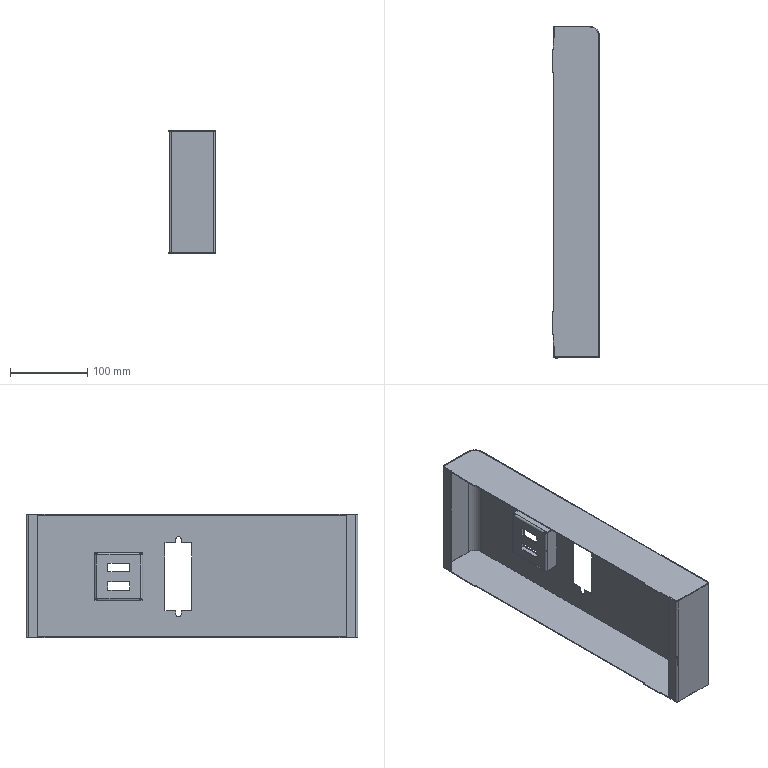Part | SolidWorks | 4 solids | 157 faces | box 61.2 x 430 x 160 mm | volume 170255 mm3 | plane 118 | cylinder 31 | spline 8 | commonest cylinder face diameters 3 x17 5.4 x7 7 x3 21.6 x2 24 x1 26.4 x1